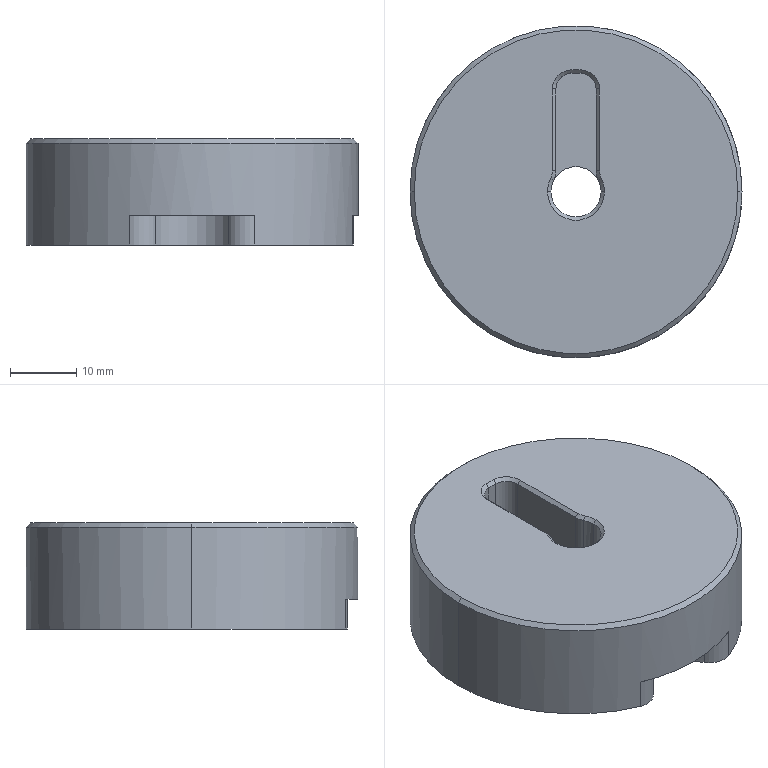NC program | NX | posted with a generic post | part box 50.292 x 50.292 x 16.057 mm
Whole program:
N10 G17 G21 G94 G90
(DRILLING_COPY_1 , TOOL : ZXZ)
N12 T01 M6
N14 G54
N16 G17 G0 G90 X13.47 Y13.47 S3000 M3
N18 G43 Z30. H1
N20 G94 G81 G98 Z-1. F200. R3.
N22 X0. Y-12.898
N24 X-13.47 Y-13.47
N26 G80
N28 G0 X-13.47 Y-13.47 Z30.
N30 M5
(FLOOR_WALL_1 , TOOL : D4)
N32 T04 M6
N34 G54
N36 G17 G0 G90 X4.162 Y28.342 S4000 M3
N38 G43 Z30. H4
N40 Z1.329
N42 G94 G1 Z-0.171 F1800.
N44 X4.655 Y26.949
N46 G3 X4.959 Y26.689 R0.4
N48 G2 X15.213 Y22.483 R27.146
N50 G1 X15.207 Y22.475
N52 G3 X9.475 Y21.472 R5.275
N54 G1 X0.193 Y12.694
N56 G2 X-0.281 Y12.898 R0.281
N58 G1 Y21.257
N60 G3 X-5.704 Y26.53 R5.275
N62 G1 X-5.706 Y26.54
N64 G2 X4.959 Y26.689 R27.146
N66 G1 X4.593 Y24.723
N68 G2 X8.844 Y23.54 R25.146
N70 G3 X8.1 Y22.925 R7.275
N72 G1 X1.719 Y16.889
N74 Y21.257
N76 G3 X0.596 Y25.139 R7.275
N78 G2 X4.593 Y24.723 R25.146
N80 G1 X4.228 Y22.757
N82 G2 X4.875 Y22.627 R23.146
N84 G1 X3.715 Y21.53
N86 G3 X3.578 Y22.868 R9.275
N88 G2 X4.228 Y22.757 R23.146
N90 G3 X4.605 Y22.89 R0.4
N92 G1 Z1.329
N94 G0 X4.162 Y28.342 Z1.135
N96 G1 Z-0.365
N98 X4.655 Y26.949
N100 G3 X4.959 Y26.689 R0.4
N102 G2 X15.213 Y22.483 R27.146
N104 G1 X15.207 Y22.475
N106 G3 X9.475 Y21.472 R5.275
N108 G1 X0.193 Y12.694
N110 G2 X-0.281 Y12.898 R0.281
N112 G1 Y21.257
N114 G3 X-5.704 Y26.53 R5.275
N116 G1 X-5.706 Y26.54
N118 G2 X4.959 Y26.689 R27.146
N120 G1 X4.593 Y24.723
N122 G2 X8.844 Y23.54 R25.146
N124 G3 X8.1 Y22.925 R7.275
N126 G1 X1.719 Y16.889
N128 Y21.257
N130 G3 X0.596 Y25.139 R7.275
N132 G2 X4.593 Y24.723 R25.146
N134 G1 X4.228 Y22.757
N136 G2 X4.875 Y22.627 R23.146
N138 G1 X3.715 Y21.53
N140 G3 X3.578 Y22.868 R9.275
N142 G2 X4.228 Y22.757 R23.146
N144 G3 X4.605 Y22.89 R0.4
N146 G1 Z1.135
N148 G0 X4.162 Y28.342 Z0.942
N150 G1 Z-0.558
N152 X4.655 Y26.949
N154 G3 X4.959 Y26.689 R0.4
N156 G2 X15.213 Y22.483 R27.146
N158 G1 X15.207 Y22.475
N160 G3 X9.475 Y21.472 R5.275
N162 G1 X0.193 Y12.694
N164 G2 X-0.281 Y12.898 R0.281
N166 G1 Y21.257
N168 G3 X-5.704 Y26.53 R5.275
N170 G1 X-5.706 Y26.54
N172 G2 X4.959 Y26.689 R27.146
N174 G1 X4.593 Y24.723
N176 G2 X8.844 Y23.54 R25.146
N178 G3 X8.1 Y22.925 R7.275
N180 G1 X1.719 Y16.889
N182 Y21.257
N184 G3 X0.596 Y25.139 R7.275
N186 G2 X4.593 Y24.723 R25.146
N188 G1 X4.228 Y22.757
N190 G2 X4.875 Y22.627 R23.146
N192 G1 X3.715 Y21.53
N194 G3 X3.578 Y22.868 R9.275
N196 G2 X4.228 Y22.757 R23.146
N198 G3 X4.605 Y22.89 R0.4
N200 G1 Z0.942
N202 G0 X4.162 Y28.342 Z0.748
N204 G1 Z-0.752
N206 X4.655 Y26.949
N208 G3 X4.959 Y26.689 R0.4
N210 G2 X15.213 Y22.483 R27.146
N212 G1 X15.207 Y22.475
N214 G3 X9.475 Y21.472 R5.275
N216 G1 X0.193 Y12.694
N218 G2 X-0.281 Y12.898 R0.281
N220 G1 Y21.257
N222 G3 X-5.704 Y26.53 R5.275
N224 G1 X-5.706 Y26.54
N226 G2 X4.959 Y26.689 R27.146
N228 G1 X4.593 Y24.723
N230 G2 X8.844 Y23.54 R25.146
N232 G3 X8.1 Y22.925 R7.275
N234 G1 X1.719 Y16.889
N236 Y21.257
N238 G3 X0.596 Y25.139 R7.275
N240 G2 X4.593 Y24.723 R25.146
N242 G1 X4.228 Y22.757
N244 G2 X4.875 Y22.627 R23.146
N246 G1 X3.715 Y21.53
N248 G3 X3.578 Y22.868 R9.275
N250 G2 X4.228 Y22.757 R23.146
N252 G3 X4.605 Y22.89 R0.4
N254 G1 Z0.748
N256 G0 X4.162 Y28.342 Z0.555
N258 G1 Z-0.945
N260 X4.655 Y26.949
N262 G3 X4.959 Y26.689 R0.4
N264 G2 X15.213 Y22.483 R27.146
N266 G1 X15.207 Y22.475
N268 G3 X9.475 Y21.472 R5.275
N270 G1 X0.193 Y12.694
N272 G2 X-0.281 Y12.898 R0.281
N274 G1 Y21.257
N276 G3 X-5.704 Y26.53 R5.275
N278 G1 X-5.706 Y26.54
N280 G2 X4.959 Y26.689 R27.146
N282 G1 X4.593 Y24.723
N284 G2 X8.844 Y23.54 R25.146
N286 G3 X8.1 Y22.925 R7.275
N288 G1 X1.719 Y16.889
N290 Y21.257
N292 G3 X0.596 Y25.139 R7.275
N294 G2 X4.593 Y24.723 R25.146
N296 G1 X4.228 Y22.757
N298 G2 X4.875 Y22.627 R23.146
N300 G1 X3.715 Y21.53
N302 G3 X3.578 Y22.868 R9.275
N304 G2 X4.228 Y22.757 R23.146
N306 G3 X4.605 Y22.89 R0.4
N308 G1 Z0.555
N310 G0 X4.162 Y28.342 Z0.361
N312 G1 Z-1.139
N314 X4.655 Y26.949
N316 G3 X4.959 Y26.689 R0.4
N318 G2 X15.213 Y22.483 R27.146
N320 G1 X15.207 Y22.475
N322 G3 X9.475 Y21.472 R5.275
N324 G1 X0.193 Y12.694
N326 G2 X-0.281 Y12.898 R0.281
N328 G1 Y21.257
N330 G3 X-5.704 Y26.53 R5.275
N332 G1 X-5.706 Y26.54
N334 G2 X4.959 Y26.689 R27.146
N336 G1 X4.593 Y24.723
N338 G2 X8.844 Y23.54 R25.146
N340 G3 X8.1 Y22.925 R7.275
N342 G1 X1.719 Y16.889
N344 Y21.257
N346 G3 X0.596 Y25.139 R7.275
N348 G2 X4.593 Y24.723 R25.146
N350 G1 X4.228 Y22.757
N352 G2 X4.875 Y22.627 R23.146
N354 G1 X3.715 Y21.53
N356 G3 X3.578 Y22.868 R9.275
N358 G2 X4.228 Y22.757 R23.146
N360 G3 X4.605 Y22.89 R0.4
N362 G1 Z0.361
N364 G0 X4.162 Y28.342 Z0.168
N366 G1 Z-1.332
N368 X4.655 Y26.949
N370 G3 X4.959 Y26.689 R0.4
N372 G2 X15.213 Y22.483 R27.146
N374 G1 X15.207 Y22.475
N376 G3 X9.475 Y21.472 R5.275
N378 G1 X0.193 Y12.694
N380 G2 X-0.281 Y12.898 R0.281
N382 G1 Y21.257
N384 G3 X-5.704 Y26.53 R5.275
N386 G1 X-5.706 Y26.54
N388 G2 X4.959 Y26.689 R27.146
N390 G1 X4.593 Y24.723
N392 G2 X8.844 Y23.54 R25.146
N394 G3 X8.1 Y22.925 R7.275
N396 G1 X1.719 Y16.889
N398 Y21.257
N400 G3 X0.596 Y25.139 R7.275
N402 G2 X4.593 Y24.723 R25.146
N404 G1 X4.228 Y22.757
N406 G2 X4.875 Y22.627 R23.146
N408 G1 X3.715 Y21.53
N410 G3 X3.578 Y22.868 R9.275
N412 G2 X4.228 Y22.757 R23.146
N414 G3 X4.605 Y22.89 R0.4
N416 G1 Z0.168
N418 G0 X4.162 Y28.342 Z-0.026
N420 G1 Z-1.526
N422 X4.655 Y26.949
N424 G3 X4.959 Y26.689 R0.4
N426 G2 X15.213 Y22.483 R27.146
N428 G1 X15.207 Y22.475
N430 G3 X9.475 Y21.472 R5.275
N432 G1 X0.193 Y12.694
N434 G2 X-0.281 Y12.898 R0.281
N436 G1 Y21.257
N438 G3 X-5.704 Y26.53 R5.275
N440 G1 X-5.706 Y26.54
N442 G2 X4.959 Y26.689 R27.146
N444 G1 X4.593 Y24.723
N446 G2 X8.844 Y23.54 R25.146
N448 G3 X8.1 Y22.925 R7.275
N450 G1 X1.719 Y16.889
N452 Y21.257
N454 G3 X0.596 Y25.139 R7.275
N456 G2 X4.593 Y24.723 R25.146
N458 G1 X4.228 Y22.757
N460 G2 X4.875 Y22.627 R23.146
N462 G1 X3.715 Y21.53
N464 G3 X3.578 Y22.868 R9.275
N466 G2 X4.228 Y22.757 R23.146
N468 G3 X4.605 Y22.89 R0.4
N470 G1 Z-0.026
N472 G0 X4.162 Y28.342 Z-0.219
N474 G1 Z-1.719
N476 X4.655 Y26.949
N478 G3 X4.959 Y26.689 R0.4
N480 G2 X15.213 Y22.483 R27.146
N482 G1 X15.207 Y22.475
N484 G3 X9.475 Y21.472 R5.275
N486 G1 X0.193 Y12.694
N488 G2 X-0.281 Y12.898 R0.281
N490 G1 Y21.257
N492 G3 X-5.704 Y26.53 R5.275
N494 G1 X-5.706 Y26.54
N496 G2 X4.959 Y26.689 R27.146
N498 G1 X4.593 Y24.723
N500 G2 X8.844 Y23.54 R25.146
N502 G3 X8.1 Y22.925 R7.275
N504 G1 X1.719 Y16.889
N506 Y21.257
N508 G3 X0.596 Y25.139 R7.275
N510 G2 X4.593 Y24.723 R25.146
N512 G1 X4.228 Y22.757
N514 G2 X4.875 Y22.627 R23.146
N516 G1 X3.715 Y21.53
N518 G3 X3.578 Y22.868 R9.275
N520 G2 X4.228 Y22.757 R23.146
N522 G3 X4.605 Y22.89 R0.4
N524 G1 Z-0.219
N526 G0 X4.162 Y28.342 Z-0.413
N528 G1 Z-1.913
N530 X4.655 Y26.949
N532 G3 X4.959 Y26.689 R0.4
N534 G2 X15.213 Y22.483 R27.146
N536 G1 X15.207 Y22.475
N538 G3 X9.475 Y21.472 R5.275
N540 G1 X0.193 Y12.694
N542 G2 X-0.281 Y12.898 R0.281
N544 G1 Y21.257
N546 G3 X-5.704 Y26.53 R5.275
N548 G1 X-5.706 Y26.54
N550 G2 X4.959 Y26.689 R27.146
N552 G1 X4.593 Y24.723
N554 G2 X8.844 Y23.54 R25.146
N556 G3 X8.1 Y22.925 R7.275
N558 G1 X1.719 Y16.889
N560 Y21.257
N562 G3 X0.596 Y25.139 R7.275
N564 G2 X4.593 Y24.723 R25.146
N566 G1 X4.228 Y22.757
N568 G2 X4.875 Y22.627 R23.146
N570 G1 X3.715 Y21.53
N572 G3 X3.578 Y22.868 R9.275
N574 G2 X4.228 Y22.757 R23.146
N576 G3 X4.605 Y22.89 R0.4
N578 G1 Z-0.413
N580 G0 X4.162 Y28.342 Z-0.606
N582 G1 Z-2.106
N584 X4.655 Y26.949
N586 G3 X4.959 Y26.689 R0.4
N588 G2 X15.213 Y22.483 R27.146
N590 G1 X15.207 Y22.475
N592 G3 X9.475 Y21.472 R5.275
N594 G1 X0.193 Y12.694
N596 G2 X-0.281 Y12.898 R0.281
N598 G1 Y21.257
N600 G3 X-5.704 Y26.53 R5.275
N602 G1 X-5.706 Y26.54
N604 G2 X4.959 Y26.689 R27.146
N606 G1 X4.593 Y24.723
N608 G2 X8.844 Y23.54 R25.146
N610 G3 X8.1 Y22.925 R7.275
N612 G1 X1.719 Y16.889
N614 Y21.257
N616 G3 X0.596 Y25.139 R7.275
N618 G2 X4.593 Y24.723 R25.146
N620 G1 X4.228 Y22.757
N622 G2 X4.875 Y22.627 R23.146
N624 G1 X3.715 Y21.53
N626 G3 X3.578 Y22.868 R9.275
N628 G2 X4.228 Y22.757 R23.146
N630 G3 X4.605 Y22.89 R0.4
N632 G1 Z-0.606
N634 G0 X4.162 Y28.342 Z-0.8
N636 G1 Z-2.3
N638 X4.655 Y26.949
N640 G3 X4.959 Y26.689 R0.4
N642 G2 X15.213 Y22.483 R27.146
N644 G1 X15.207 Y22.475
N646 G3 X9.475 Y21.472 R5.275
N648 G1 X0.193 Y12.694
N650 G2 X-0.281 Y12.898 R0.281
N652 G1 Y21.257
N654 G3 X-5.704 Y26.53 R5.275
N656 G1 X-5.706 Y26.54
N658 G2 X4.959 Y26.689 R27.146
N660 G1 X4.593 Y24.723
N662 G2 X8.844 Y23.54 R25.146
N664 G3 X8.1 Y22.925 R7.275
N666 G1 X1.719 Y16.889
N668 Y21.257
N670 G3 X0.596 Y25.139 R7.275
N672 G2 X4.593 Y24.723 R25.146
N674 G1 X4.228 Y22.757
N676 G2 X4.875 Y22.627 R23.146
N678 G1 X3.715 Y21.53
N680 G3 X3.578 Y22.868 R9.275
N682 G2 X4.228 Y22.757 R23.146
N684 G3 X4.605 Y22.89 R0.4
N686 G1 Z-0.8
N688 G0 X4.162 Y28.342 Z-0.993
N690 G1 Z-2.493
N692 X4.655 Y26.949
N694 G3 X4.959 Y26.689 R0.4
N696 G2 X15.213 Y22.483 R27.146
N698 G1 X15.207 Y22.475
N700 G3 X9.475 Y21.472 R5.275
N702 G1 X0.193 Y12.694
N704 G2 X-0.281 Y12.898 R0.281
N706 G1 Y21.257
N708 G3 X-5.704 Y26.53 R5.275
N710 G1 X-5.706 Y26.54
N712 G2 X4.959 Y26.689 R27.146
N714 G1 X4.593 Y24.723
N716 G2 X8.844 Y23.54 R25.146
N718 G3 X8.1 Y22.925 R7.275
N720 G1 X1.719 Y16.889
N722 Y21.257
N724 G3 X0.596 Y25.139 R7.275
N726 G2 X4.593 Y24.723 R25.146
N728 G1 X4.228 Y22.757
N730 G2 X4.875 Y22.627 R23.146
N732 G1 X3.715 Y21.53
N734 G3 X3.578 Y22.868 R9.275
N736 G2 X4.228 Y22.757 R23.146
N738 G3 X4.605 Y22.89 R0.4
N740 G1 Z-0.993
N742 G0 X4.162 Y28.342 Z-1.187
N744 G1 Z-2.687
N746 X4.655 Y26.949
N748 G3 X4.959 Y26.689 R0.4
N750 G2 X15.213 Y22.483 R27.146
N752 G1 X15.207 Y22.475
N754 G3 X9.475 Y21.472 R5.275
N756 G1 X0.193 Y12.694
N758 G2 X-0.281 Y12.898 R0.281
N760 G1 Y21.257
N762 G3 X-5.704 Y26.53 R5.275
N764 G1 X-5.706 Y26.54
N766 G2 X4.959 Y26.689 R27.146
N768 G1 X4.593 Y24.723
N770 G2 X8.844 Y23.54 R25.146
N772 G3 X8.1 Y22.925 R7.275
N774 G1 X1.719 Y16.889
N776 Y21.257
N778 G3 X0.596 Y25.139 R7.275
N780 G2 X4.593 Y24.723 R25.146
N782 G1 X4.228 Y22.757
N784 G2 X4.875 Y22.627 R23.146
N786 G1 X3.715 Y21.53
N788 G3 X3.578 Y22.868 R9.275
N790 G2 X4.228 Y22.757 R23.146
N792 G3 X4.605 Y22.89 R0.4
N794 G1 Z-1.187
N796 G0 X4.162 Y28.342 Z-1.38
N798 G1 Z-2.88
N800 X4.655 Y26.949
N802 G3 X4.959 Y26.689 R0.4
N804 G2 X15.213 Y22.483 R27.146
N806 G1 X15.207 Y22.475
N808 G3 X9.475 Y21.472 R5.275
N810 G1 X0.193 Y12.694
N812 G2 X-0.281 Y12.898 R0.281
N814 G1 Y21.257
N816 G3 X-5.704 Y26.53 R5.275
N818 G1 X-5.706 Y26.54
N820 G2 X4.959 Y26.689 R27.146
N822 G1 X4.593 Y24.723
N824 G2 X8.844 Y23.54 R25.146
N826 G3 X8.1 Y22.925 R7.275
N828 G1 X1.719 Y16.889
N830 Y21.257
N832 G3 X0.596 Y25.139 R7.275
N834 G2 X4.593 Y24.723 R25.146
N836 G1 X4.228 Y22.757
N838 G2 X4.875 Y22.627 R23.146
N840 G1 X3.715 Y21.53
N842 G3 X3.578 Y22.868 R9.275
N844 G2 X4.228 Y22.757 R23.146
N846 G3 X4.605 Y22.89 R0.4
N848 G1 Z-1.38
N850 G0 X4.162 Y28.342 Z-1.574
N852 G1 Z-3.074
N854 X4.655 Y26.949
N856 G3 X4.959 Y26.689 R0.4
N858 G2 X15.213 Y22.483 R27.146
N860 G1 X15.207 Y22.475
N862 G3 X9.475 Y21.472 R5.275
N864 G1 X0.193 Y12.694
N866 G2 X-0.281 Y12.898 R0.281
N868 G1 Y21.257
N870 G3 X-5.704 Y26.53 R5.275
N872 G1 X-5.706 Y26.54
N874 G2 X4.959 Y26.689 R27.146
N876 G1 X4.593 Y24.723
N878 G2 X8.844 Y23.54 R25.146
N880 G3 X8.1 Y22.925 R7.275
N882 G1 X1.719 Y16.889
N884 Y21.257
N886 G3 X0.596 Y25.139 R7.275
N888 G2 X4.593 Y24.723 R25.146
N890 G1 X4.228 Y22.757
N892 G2 X4.875 Y22.627 R23.146
N894 G1 X3.715 Y21.53
N896 G3 X3.578 Y22.868 R9.275
N898 G2 X4.228 Y22.757 R23.146
N900 G3 X4.605 Y22.89 R0.4
N902 G1 Z-1.574
N904 G0 X4.162 Y28.342 Z-1.767
N906 G1 Z-3.267
N908 X4.655 Y26.949
N910 G3 X4.959 Y26.689 R0.4
N912 G2 X15.213 Y22.483 R27.146
N914 G1 X15.207 Y22.475
N916 G3 X9.475 Y21.472 R5.275
N918 G1 X0.193 Y12.694
N920 G2 X-0.281 Y12.898 R0.281
N922 G1 Y21.257
N924 G3 X-5.704 Y26.53 R5.275
N926 G1 X-5.706 Y26.54
N928 G2 X4.959 Y26.689 R27.146
N930 G1 X4.593 Y24.723
N932 G2 X8.844 Y23.54 R25.146
N934 G3 X8.1 Y22.925 R7.275
N936 G1 X1.719 Y16.889
N938 Y21.257
N940 G3 X0.596 Y25.139 R7.275
N942 G2 X4.593 Y24.723 R25.146
N944 G1 X4.228 Y22.757
N946 G2 X4.875 Y22.627 R23.146
N948 G1 X3.715 Y21.53
N950 G3 X3.578 Y22.868 R9.275
N952 G2 X4.228 Y22.757 R23.146
N954 G3 X4.605 Y22.89 R0.4
N956 G1 Z-1.767
N958 G0 X4.162 Y28.342 Z-1.961
N960 G1 Z-3.461
N962 X4.655 Y26.949
N964 G3 X4.959 Y26.689 R0.4
N966 G2 X15.213 Y22.483 R27.146
N968 G1 X15.207 Y22.475
N970 G3 X9.475 Y21.472 R5.275
N972 G1 X0.193 Y12.694
N974 G2 X-0.281 Y12.898 R0.281
N976 G1 Y21.257
N978 G3 X-5.704 Y26.53 R5.275
N980 G1 X-5.706 Y26.54
N982 G2 X4.959 Y26.689 R27.146
N984 G1 X4.593 Y24.723
N986 G2 X8.844 Y23.54 R25.146
N988 G3 X8.1 Y22.925 R7.275
N990 G1 X1.719 Y16.889
N992 Y21.257
N994 G3 X0.596 Y25.139 R7.275
N996 G2 X4.593 Y24.723 R25.146
N998 G1 X4.228 Y22.757
N1000 G2 X4.875 Y22.627 R23.146
N1002 G1 X3.715 Y21.53
N1004 G3 X3.578 Y22.868 R9.275
N1006 G2 X4.228 Y22.757 R23.146
N1008 G3 X4.605 Y22.89 R0.4
N1010 G1 Z-1.961
N1012 G0 X4.162 Y28.342 Z-2.154
N1014 G1 Z-3.654
N1016 X4.655 Y26.949
N1018 G3 X4.959 Y26.689 R0.4
N1020 G2 X15.213 Y22.483 R27.146
N1022 G1 X15.207 Y22.475
N1024 G3 X9.475 Y21.472 R5.275
N1026 G1 X0.193 Y12.694
N1028 G2 X-0.281 Y12.898 R0.281
N1030 G1 Y21.257
N1032 G3 X-5.704 Y26.53 R5.275
N1034 G1 X-5.706 Y26.54
N1036 G2 X4.959 Y26.689 R27.146
N1038 G1 X4.593 Y24.723
N1040 G2 X8.844 Y23.54 R25.146
N1042 G3 X8.1 Y22.925 R7.275
N1044 G1 X1.719 Y16.889
N1046 Y21.257
N1048 G3 X0.596 Y25.139 R7.275
N1050 G2 X4.593 Y24.723 R25.146
N1052 G1 X4.228 Y22.757
N1054 G2 X4.875 Y22.627 R23.146
N1056 G1 X3.715 Y21.53
N1058 G3 X3.578 Y22.868 R9.275
N1060 G2 X4.228 Y22.757 R23.146
N1062 G3 X4.605 Y22.89 R0.4
N1064 G1 Z-2.154
N1066 G0 X4.162 Y28.342 Z-2.348
N1068 G1 Z-3.848
N1070 X4.655 Y26.949
N1072 G3 X4.959 Y26.689 R0.4
N1074 G2 X15.213 Y22.483 R27.146
N1076 G1 X15.207 Y22.475
N1078 G3 X9.475 Y21.472 R5.275
N1080 G1 X0.193 Y12.694
N1082 G2 X-0.281 Y12.898 R0.281
N1084 G1 Y21.257
N1086 G3 X-5.704 Y26.53 R5.275
N1088 G1 X-5.706 Y26.54
N1090 G2 X4.959 Y26.689 R27.146
N1092 G1 X4.593 Y24.723
N1094 G2 X8.844 Y23.54 R25.146
N1096 G3 X8.1 Y22.925 R7.275
N1098 G1 X1.719 Y16.889
N1100 Y21.257
N1102 G3 X0.596 Y25.139 R7.275
N1104 G2 X4.593 Y24.723 R25.146
N1106 G1 X4.228 Y22.757
N1108 G2 X4.875 Y22.627 R23.146
N1110 G1 X3.715 Y21.53
N1112 G3 X3.578 Y22.868 R9.275
N1114 G2 X4.228 Y22.757 R23.146
N1116 G3 X4.605 Y22.89 R0.4
N1118 G1 Z-2.348
N1120 G0 X4.162 Y28.342 Z-2.541
N1122 G1 Z-4.041
N1124 X4.655 Y26.949
N1126 G3 X4.959 Y26.689 R0.4
N1128 G2 X15.213 Y22.483 R27.146
N1130 G1 X15.207 Y22.475
N1132 G3 X9.475 Y21.472 R5.275
N1134 G1 X0.193 Y12.694
N1136 G2 X-0.281 Y12.898 R0.281
N1138 G1 Y21.257
N1140 G3 X-5.704 Y26.53 R5.275
N1142 G1 X-5.706 Y26.54
N1144 G2 X4.959 Y26.689 R27.146
N1146 G1 X4.593 Y24.723
N1148 G2 X8.844 Y23.54 R25.146
N1150 G3 X8.1 Y22.925 R7.275
N1152 G1 X1.719 Y16.889
N1154 Y21.257
N1156 G3 X0.596 Y25.139 R7.275
N1158 G2 X4.593 Y24.723 R25.146
N1160 G1 X4.228 Y22.757
N1162 G2 X4.875 Y22.627 R23.146
N1164 G1 X3.715 Y21.53
N1166 G3 X3.578 Y22.868 R9.275
N1168 G2 X4.228 Y22.757 R23.146
N1170 G3 X4.605 Y22.89 R0.4
N1172 G1 Z-2.541
N1174 G0 X4.162 Y28.342 Z-2.735
N1176 G1 Z-4.235
N1178 X4.655 Y26.949
N1180 G3 X4.959 Y26.689 R0.4
N1182 G2 X15.213 Y22.483 R27.146
N1184 G1 X15.207 Y22.475
N1186 G3 X9.475 Y21.472 R5.275
N1188 G1 X0.193 Y12.694
N1190 G2 X-0.281 Y12.898 R0.281
N1192 G1 Y21.257
N1194 G3 X-5.704 Y26.53 R5.275
N1196 G1 X-5.706 Y26.54
N1198 G2 X4.959 Y26.689 R27.146
N1200 G1 X4.593 Y24.723
N1202 G2 X8.844 Y23.54 R25.146
N1204 G3 X8.1 Y22.925 R7.275
N1206 G1 X1.719 Y16.889
N1208 Y21.257
N1210 G3 X0.596 Y25.139 R7.275
N1212 G2 X4.593 Y24.723 R25.146
N1214 G1 X4.228 Y22.757
N1216 G2 X4.875 Y22.627 R23.146
N1218 G1 X3.715 Y21.53
N1220 G3 X3.578 Y22.868 R9.275
N1222 G2 X4.228 Y22.757 R23.146
N1224 G3 X4.605 Y22.89 R0.4
N1226 G1 Z-2.735
N1228 G0 X4.162 Y28.342 Z-2.928
N1230 G1 Z-4.428
N1232 X4.655 Y26.949
N1234 G3 X4.959 Y26.689 R0.4
N1236 G2 X15.213 Y22.483 R27.146
N1238 G1 X15.207 Y22.475
N1240 G3 X9.475 Y21.472 R5.275
N1242 G1 X0.193 Y12.694
N1244 G2 X-0.281 Y12.898 R0.281
N1246 G1 Y21.257
N1248 G3 X-5.704 Y26.53 R5.275
N1250 G1 X-5.706 Y26.54
N1252 G2 X4.959 Y26.689 R27.146
N1254 G1 X4.593 Y24.723
N1256 G2 X8.844 Y23.54 R25.146
N1258 G3 X8.1 Y22.925 R7.275
N1260 G1 X1.719 Y16.889
N1262 Y21.257
N1264 G3 X0.596 Y25.139 R7.275
N1266 G2 X4.593 Y24.723 R25.146
N1268 G1 X4.228 Y22.757
N1270 G2 X4.875 Y22.627 R23.146
N1272 G1 X3.715 Y21.53
N1274 G3 X3.578 Y22.868 R9.275
N1276 G2 X4.228 Y22.757 R23.146
N1278 G3 X4.605 Y22.89 R0.4
N1280 G1 Z-2.928
N1282 G0 Z30.
N1284 X-28.625 Y-1.085
N1286 Z1.329
N1288 G1 Z-0.171
N1290 X-27.346 Y-0.346
N1292 G3 X-27.146 Y0. R0.4
N1294 G2 X-25.574 Y9.104 R27.146
N1296 G1 X-25.565 Y9.1
N1298 G3 X-22.973 Y3.69 R5.275
N1300 G2 X-22.973 Y-3.69 R4.25
N1302 G3 X-25.565 Y-9.1 R5.275
N1304 G1 X-25.574 Y-9.104
N1306 G2 X-27.146 Y0. R27.146
N1308 G1 X-25.146
N1310 G2 X-25.004 Y2.673 R25.146
N1312 G3 X-23.966 Y1.953 R7.275
N1314 G2 X-23.966 Y-1.953 R2.25
N1316 G3 X-25.004 Y-2.673 R7.275
N1318 G2 X-25.146 Y0. R25.146
N1320 G3 X-25.346 Y0.346 R0.4
N1322 G1 X-28.643 Y0.391
N1324 Z1.329
N1326 G0 X-28.625 Y-1.085 Z1.135
N1328 G1 Z-0.365
N1330 X-27.346 Y-0.346
N1332 G3 X-27.146 Y0. R0.4
N1334 G2 X-25.574 Y9.104 R27.146
N1336 G1 X-25.565 Y9.1
N1338 G3 X-22.973 Y3.69 R5.275
N1340 G2 X-22.973 Y-3.69 R4.25
N1342 G3 X-25.565 Y-9.1 R5.275
N1344 G1 X-25.574 Y-9.104
N1346 G2 X-27.146 Y0. R27.146
N1348 G1 X-25.146
N1350 G2 X-25.004 Y2.673 R25.146
N1352 G3 X-23.966 Y1.953 R7.275
N1354 G2 X-23.966 Y-1.953 R2.25
N1356 G3 X-25.004 Y-2.673 R7.275
N1358 G2 X-25.146 Y0. R25.146
N1360 G3 X-25.346 Y0.346 R0.4
N1362 G1 X-28.643 Y0.391
N1364 Z1.135
N1366 G0 X-28.625 Y-1.085 Z0.942
N1368 G1 Z-0.558
N1370 X-27.346 Y-0.346
N1372 G3 X-27.146 Y0. R0.4
N1374 G2 X-25.574 Y9.104 R27.146
N1376 G1 X-25.565 Y9.1
N1378 G3 X-22.973 Y3.69 R5.275
N1380 G2 X-22.973 Y-3.69 R4.25
N1382 G3 X-25.565 Y-9.1 R5.275
N1384 G1 X-25.574 Y-9.104
N1386 G2 X-27.146 Y0. R27.146
N1388 G1 X-25.146
N1390 G2 X-25.004 Y2.673 R25.146
N1392 G3 X-23.966 Y1.953 R7.275
N1394 G2 X-23.966 Y-1.953 R2.25
N1396 G3 X-25.004 Y-2.673 R7.275
N1398 G2 X-25.146 Y0. R25.146
N1400 G3 X-25.346 Y0.346 R0.4
N1402 G1 X-28.643 Y0.391
N1404 Z0.942
N1406 G0 X-28.625 Y-1.085 Z0.748
N1408 G1 Z-0.752
N1410 X-27.346 Y-0.346
N1412 G3 X-27.146 Y0. R0.4
N1414 G2 X-25.574 Y9.104 R27.146
N1416 G1 X-25.565 Y9.1
N1418 G3 X-22.973 Y3.69 R5.275
N1420 G2 X-22.973 Y-3.69 R4.25
N1422 G3 X-25.565 Y-9.1 R5.275
N1424 G1 X-25.574 Y-9.104
N1426 G2 X-27.146 Y0. R27.146
N1428 G1 X-25.146
N1430 G2 X-25.004 Y2.673 R25.146
N1432 G3 X-23.966 Y1.953 R7.275
N1434 G2 X-23.966 Y-1.953 R2.25
N1436 G3 X-25.004 Y-2.673 R7.275
N1438 G2 X-25.146 Y0. R25.146
N1440 G3 X-25.346 Y0.346 R0.4
N1442 G1 X-28.643 Y0.391
N1444 Z0.748
N1446 G0 X-28.625 Y-1.085 Z0.555
N1448 G1 Z-0.945
N1450 X-27.346 Y-0.346
N1452 G3 X-27.146 Y0. R0.4
N1454 G2 X-25.574 Y9.104 R27.146
N1456 G1 X-25.565 Y9.1
N1458 G3 X-22.973 Y3.69 R5.275
N1460 G2 X-22.973 Y-3.69 R4.25
N1462 G3 X-25.565 Y-9.1 R5.275
N1464 G1 X-25.574 Y-9.104
N1466 G2 X-27.146 Y0. R27.146
N1468 G1 X-25.146
N1470 G2 X-25.004 Y2.673 R25.146
N1472 G3 X-23.966 Y1.953 R7.275
N1474 G2 X-23.966 Y-1.953 R2.25
N1476 G3 X-25.004 Y-2.673 R7.275
N1478 G2 X-25.146 Y0. R25.146
N1480 G3 X-25.346 Y0.346 R0.4
N1482 G1 X-28.643 Y0.391
N1484 Z0.555
N1486 G0 X-28.625 Y-1.085 Z0.361
N1488 G1 Z-1.139
N1490 X-27.346 Y-0.346
N1492 G3 X-27.146 Y0. R0.4
N1494 G2 X-25.574 Y9.104 R27.146
N1496 G1 X-25.565 Y9.1
N1498 G3 X-22.973 Y3.69 R5.275
N1500 G2 X-22.973 Y-3.69 R4.25
N1502 G3 X-25.565 Y-9.1 R5.275
N1504 G1 X-25.574 Y-9.104
N1506 G2 X-27.146 Y0. R27.146
N1508 G1 X-25.146
N1510 G2 X-25.004 Y2.673 R25.146
N1512 G3 X-23.966 Y1.953 R7.275
N1514 G2 X-23.966 Y-1.953 R2.25
N1516 G3 X-25.004 Y-2.673 R7.275
N1518 G2 X-25.146 Y0. R25.146
N1520 G3 X-25.346 Y0.346 R0.4
N1522 G1 X-28.643 Y0.391
N1524 Z0.361
N1526 G0 X-28.625 Y-1.085 Z0.168
N1528 G1 Z-1.332
N1530 X-27.346 Y-0.346
N1532 G3 X-27.146 Y0. R0.4
N1534 G2 X-25.574 Y9.104 R27.146
N1536 G1 X-25.565 Y9.1
N1538 G3 X-22.973 Y3.69 R5.275
N1540 G2 X-22.973 Y-3.69 R4.25
N1542 G3 X-25.565 Y-9.1 R5.275
N1544 G1 X-25.574 Y-9.104
N1546 G2 X-27.146 Y0. R27.146
N1548 G1 X-25.146
N1550 G2 X-25.004 Y2.673 R25.146
N1552 G3 X-23.966 Y1.953 R7.275
N1554 G2 X-23.966 Y-1.953 R2.25
N1556 G3 X-25.004 Y-2.673 R7.275
N1558 G2 X-25.146 Y0. R25.146
N1560 G3 X-25.346 Y0.346 R0.4
N1562 G1 X-28.643 Y0.391
N1564 Z0.168
N1566 G0 X-28.625 Y-1.085 Z-0.026
N1568 G1 Z-1.526
N1570 X-27.346 Y-0.346
N1572 G3 X-27.146 Y0. R0.4
N1574 G2 X-25.574 Y9.104 R27.146
N1576 G1 X-25.565 Y9.1
N1578 G3 X-22.973 Y3.69 R5.275
N1580 G2 X-22.973 Y-3.69 R4.25
N1582 G3 X-25.565 Y-9.1 R5.275
N1584 G1 X-25.574 Y-9.104
N1586 G2 X-27.146 Y0. R27.146
N1588 G1 X-25.146
N1590 G2 X-25.004 Y2.673 R25.146
N1592 G3 X-23.966 Y1.953 R7.275
N1594 G2 X-23.966 Y-1.953 R2.25
N1596 G3 X-25.004 Y-2.673 R7.275
N1598 G2 X-25.146 Y0. R25.146
N1600 G3 X-25.346 Y0.346 R0.4
N1602 G1 X-28.643 Y0.391
N1604 Z-0.026
N1606 G0 X-28.625 Y-1.085 Z-0.219
N1608 G1 Z-1.719
N1610 X-27.346 Y-0.346
N1612 G3 X-27.146 Y0. R0.4
N1614 G2 X-25.574 Y9.104 R27.146
N1616 G1 X-25.565 Y9.1
N1618 G3 X-22.973 Y3.69 R5.275
N1620 G2 X-22.973 Y-3.69 R4.25
N1622 G3 X-25.565 Y-9.1 R5.275
N1624 G1 X-25.574 Y-9.104
N1626 G2 X-27.146 Y0. R27.146
N1628 G1 X-25.146
N1630 G2 X-25.004 Y2.673 R25.146
N1632 G3 X-23.966 Y1.953 R7.275
N1634 G2 X-23.966 Y-1.953 R2.25
N1636 G3 X-25.004 Y-2.673 R7.275
N1638 G2 X-25.146 Y0. R25.146
N1640 G3 X-25.346 Y0.346 R0.4
N1642 G1 X-28.643 Y0.391
N1644 Z-0.219
N1646 G0 X-28.625 Y-1.085 Z-0.413
N1648 G1 Z-1.913
N1650 X-27.346 Y-0.346
N1652 G3 X-27.146 Y0. R0.4
N1654 G2 X-25.574 Y9.104 R27.146
N1656 G1 X-25.565 Y9.1
N1658 G3 X-22.973 Y3.69 R5.275
N1660 G2 X-22.973 Y-3.69 R4.25
N1662 G3 X-25.565 Y-9.1 R5.275
N1664 G1 X-25.574 Y-9.104
N1666 G2 X-27.146 Y0. R27.146
N1668 G1 X-25.146
N1670 G2 X-25.004 Y2.673 R25.146
N1672 G3 X-23.966 Y1.953 R7.275
N1674 G2 X-23.966 Y-1.953 R2.25
N1676 G3 X-25.004 Y-2.673 R7.275
N1678 G2 X-25.146 Y0. R25.146
N1680 G3 X-25.346 Y0.346 R0.4
N1682 G1 X-28.643 Y0.391
N1684 Z-0.413
N1686 G0 X-28.625 Y-1.085 Z-0.606
N1688 G1 Z-2.106
N1690 X-27.346 Y-0.346
N1692 G3 X-27.146 Y0. R0.4
N1694 G2 X-25.574 Y9.104 R27.146
N1696 G1 X-25.565 Y9.1
N1698 G3 X-22.973 Y3.69 R5.275
N1700 G2 X-22.973 Y-3.69 R4.25
N1702 G3 X-25.565 Y-9.1 R5.275
N1704 G1 X-25.574 Y-9.104
N1706 G2 X-27.146 Y0. R27.146
N1708 G1 X-25.146
N1710 G2 X-25.004 Y2.673 R25.146
N1712 G3 X-23.966 Y1.953 R7.275
N1714 G2 X-23.966 Y-1.953 R2.25
N1716 G3 X-25.004 Y-2.673 R7.275
N1718 G2 X-25.146 Y0. R25.146
N1720 G3 X-25.346 Y0.346 R0.4
N1722 G1 X-28.643 Y0.391
N1724 Z-0.606
N1726 G0 X-28.625 Y-1.085 Z-0.8
N1728 G1 Z-2.3
N1730 X-27.346 Y-0.346
N1732 G3 X-27.146 Y0. R0.4
N1734 G2 X-25.574 Y9.104 R27.146
N1736 G1 X-25.565 Y9.1
N1738 G3 X-22.973 Y3.69 R5.275
N1740 G2 X-22.973 Y-3.69 R4.25
N1742 G3 X-25.565 Y-9.1 R5.275
N1744 G1 X-25.574 Y-9.104
N1746 G2 X-27.146 Y0. R27.146
N1748 G1 X-25.146
N1750 G2 X-25.004 Y2.673 R25.146
N1752 G3 X-23.966 Y1.953 R7.275
N1754 G2 X-23.966 Y-1.953 R2.25
N1756 G3 X-25.004 Y-2.673 R7.275
N1758 G2 X-25.146 Y0. R25.146
N1760 G3 X-25.346 Y0.346 R0.4
N1762 G1 X-28.643 Y0.391
N1764 Z-0.8
N1766 G0 X-28.625 Y-1.085 Z-0.993
N1768 G1 Z-2.493
N1770 X-27.346 Y-0.346
N1772 G3 X-27.146 Y0. R0.4
N1774 G2 X-25.574 Y9.104 R27.146
N1776 G1 X-25.565 Y9.1
N1778 G3 X-22.973 Y3.69 R5.275
N1780 G2 X-22.973 Y-3.69 R4.25
N1782 G3 X-25.565 Y-9.1 R5.275
N1784 G1 X-25.574 Y-9.104
N1786 G2 X-27.146 Y0. R27.146
N1788 G1 X-25.146
N1790 G2 X-25.004 Y2.673 R25.146
N1792 G3 X-23.966 Y1.953 R7.275
N1794 G2 X-23.966 Y-1.953 R2.25
N1796 G3 X-25.004 Y-2.673 R7.275
N1798 G2 X-25.146 Y0. R25.146
N1800 G3 X-25.346 Y0.346 R0.4
N1802 G1 X-28.643 Y0.391
N1804 Z-0.993
N1806 G0 X-28.625 Y-1.085 Z-1.187
N1808 G1 Z-2.687
N1810 X-27.346 Y-0.346
N1812 G3 X-27.146 Y0. R0.4
N1814 G2 X-25.574 Y9.104 R27.146
N1816 G1 X-25.565 Y9.1
N1818 G3 X-22.973 Y3.69 R5.275
N1820 G2 X-22.973 Y-3.69 R4.25
N1822 G3 X-25.565 Y-9.1 R5.275
N1824 G1 X-25.574 Y-9.104
N1826 G2 X-27.146 Y0. R27.146
N1828 G1 X-25.146
N1830 G2 X-25.004 Y2.673 R25.146
N1832 G3 X-23.966 Y1.953 R7.275
N1834 G2 X-23.966 Y-1.953 R2.25
N1836 G3 X-25.004 Y-2.673 R7.275
N1838 G2 X-25.146 Y0. R25.146
N1840 G3 X-25.346 Y0.346 R0.4
N1842 G1 X-28.643 Y0.391
N1844 Z-1.187
N1846 G0 X-28.625 Y-1.085 Z-1.38
N1848 G1 Z-2.88
N1850 X-27.346 Y-0.346
N1852 G3 X-27.146 Y0. R0.4
N1854 G2 X-25.574 Y9.104 R27.146
N1856 G1 X-25.565 Y9.1
N1858 G3 X-22.973 Y3.69 R5.275
N1860 G2 X-22.973 Y-3.69 R4.25
N1862 G3 X-25.565 Y-9.1 R5.275
N1864 G1 X-25.574 Y-9.104
N1866 G2 X-27.146 Y0. R27.146
N1868 G1 X-25.146
N1870 G2 X-25.004 Y2.673 R25.146
N1872 G3 X-23.966 Y1.953 R7.275
N1874 G2 X-23.966 Y-1.953 R2.25
N1876 G3 X-25.004 Y-2.673 R7.275
N1878 G2 X-25.146 Y0. R25.146
N1880 G3 X-25.346 Y0.346 R0.4
N1882 G1 X-28.643 Y0.391
N1884 Z-1.38
N1886 G0 X-28.625 Y-1.085 Z-1.574
N1888 G1 Z-3.074
N1890 X-27.346 Y-0.346
N1892 G3 X-27.146 Y0. R0.4
N1894 G2 X-25.574 Y9.104 R27.146
N1896 G1 X-25.565 Y9.1
N1898 G3 X-22.973 Y3.69 R5.275
N1900 G2 X-22.973 Y-3.69 R4.25
N1902 G3 X-25.565 Y-9.1 R5.275
N1904 G1 X-25.574 Y-9.104
N1906 G2 X-27.146 Y0. R27.146
N1908 G1 X-25.146
N1910 G2 X-25.004 Y2.673 R25.146
N1912 G3 X-23.966 Y1.953 R7.275
N1914 G2 X-23.966 Y-1.953 R2.25
N1916 G3 X-25.004 Y-2.673 R7.275
N1918 G2 X-25.146 Y0. R25.146
N1920 G3 X-25.346 Y0.346 R0.4
N1922 G1 X-28.643 Y0.391
N1924 Z-1.574
N1926 G0 X-28.625 Y-1.085 Z-1.767
N1928 G1 Z-3.267
N1930 X-27.346 Y-0.346
N1932 G3 X-27.146 Y0. R0.4
N1934 G2 X-25.574 Y9.104 R27.146
N1936 G1 X-25.565 Y9.1
N1938 G3 X-22.973 Y3.69 R5.275
N1940 G2 X-22.973 Y-3.69 R4.25
N1942 G3 X-25.565 Y-9.1 R5.275
N1944 G1 X-25.574 Y-9.104
N1946 G2 X-27.146 Y0. R27.146
N1948 G1 X-25.146
N1950 G2 X-25.004 Y2.673 R25.146
N1952 G3 X-23.966 Y1.953 R7.275
N1954 G2 X-23.966 Y-1.953 R2.25
N1956 G3 X-25.004 Y-2.673 R7.275
N1958 G2 X-25.146 Y0. R25.146
N1960 G3 X-25.346 Y0.346 R0.4
N1962 G1 X-28.643 Y0.391
N1964 Z-1.767
N1966 G0 X-28.625 Y-1.085 Z-1.961
N1968 G1 Z-3.461
N1970 X-27.346 Y-0.346
N1972 G3 X-27.146 Y0. R0.4
N1974 G2 X-25.574 Y9.104 R27.146
N1976 G1 X-25.565 Y9.1
N1978 G3 X-22.973 Y3.69 R5.275
N1980 G2 X-22.973 Y-3.69 R4.25
N1982 G3 X-25.565 Y-9.1 R5.275
N1984 G1 X-25.574 Y-9.104
N1986 G2 X-27.146 Y0. R27.146
N1988 G1 X-25.146
N1990 G2 X-25.004 Y2.673 R25.146
N1992 G3 X-23.966 Y1.953 R7.275
N1994 G2 X-23.966 Y-1.953 R2.25
N1996 G3 X-25.004 Y-2.673 R7.275
N1998 G2 X-25.146 Y0. R25.146
N2000 G3 X-25.346 Y0.346 R0.4
N2002 G1 X-28.643 Y0.391
N2004 Z-1.961
N2006 G0 X-28.625 Y-1.085 Z-2.154
N2008 G1 Z-3.654
N2010 X-27.346 Y-0.346
N2012 G3 X-27.146 Y0. R0.4
N2014 G2 X-25.574 Y9.104 R27.146
N2016 G1 X-25.565 Y9.1
N2018 G3 X-22.973 Y3.69 R5.275
N2020 G2 X-22.973 Y-3.69 R4.25
N2022 G3 X-25.565 Y-9.1 R5.275
N2024 G1 X-25.574 Y-9.104
N2026 G2 X-27.146 Y0. R27.146
N2028 G1 X-25.146
N2030 G2 X-25.004 Y2.673 R25.146
N2032 G3 X-23.966 Y1.953 R7.275
N2034 G2 X-23.966 Y-1.953 R2.25
N2036 G3 X-25.004 Y-2.673 R7.275
N2038 G2 X-25.146 Y0. R25.146
N2040 G3 X-25.346 Y0.346 R0.4
N2042 G1 X-28.643 Y0.391
N2044 Z-2.154
N2046 G0 X-28.625 Y-1.085 Z-2.348
N2048 G1 Z-3.848
N2050 X-27.346 Y-0.346
N2052 G3 X-27.146 Y0. R0.4
N2054 G2 X-25.574 Y9.104 R27.146
N2056 G1 X-25.565 Y9.1
N2058 G3 X-22.973 Y3.69 R5.275
N2060 G2 X-22.973 Y-3.69 R4.25
N2062 G3 X-25.565 Y-9.1 R5.275
N2064 G1 X-25.574 Y-9.104
N2066 G2 X-27.146 Y0. R27.146
N2068 G1 X-25.146
N2070 G2 X-25.004 Y2.673 R25.146
N2072 G3 X-23.966 Y1.953 R7.275
N2074 G2 X-23.966 Y-1.953 R2.25
N2076 G3 X-25.004 Y-2.673 R7.275
N2078 G2 X-25.146 Y0. R25.146
N2080 G3 X-25.346 Y0.346 R0.4
N2082 G1 X-28.643 Y0.391
N2084 Z-2.348
N2086 G0 X-28.625 Y-1.085 Z-2.541
N2088 G1 Z-4.041
N2090 X-27.346 Y-0.346
N2092 G3 X-27.146 Y0. R0.4
N2094 G2 X-25.574 Y9.104 R27.146
N2096 G1 X-25.565 Y9.1
N2098 G3 X-22.973 Y3.69 R5.275
N2100 G2 X-22.973 Y-3.69 R4.25
N2102 G3 X-25.565 Y-9.1 R5.275
N2104 G1 X-25.574 Y-9.104
N2106 G2 X-27.146 Y0. R27.146
N2108 G1 X-25.146
N2110 G2 X-25.004 Y2.673 R25.146
N2112 G3 X-23.966 Y1.953 R7.275
N2114 G2 X-23.966 Y-1.953 R2.25
N2116 G3 X-25.004 Y-2.673 R7.275
N2118 G2 X-25.146 Y0. R25.146
N2120 G3 X-25.346 Y0.346 R0.4
N2122 G1 X-28.643 Y0.391
N2124 Z-2.541
N2126 G0 X-28.625 Y-1.085 Z-2.735
N2128 G1 Z-4.235
N2130 X-27.346 Y-0.346
N2132 G3 X-27.146 Y0. R0.4
N2134 G2 X-25.574 Y9.104 R27.146
N2136 G1 X-25.565 Y9.1
N2138 G3 X-22.973 Y3.69 R5.275
N2140 G2 X-22.973 Y-3.69 R4.25
N2142 G3 X-25.565 Y-9.1 R5.275
N2144 G1 X-25.574 Y-9.104
N2146 G2 X-27.146 Y0. R27.146
N2148 G1 X-25.146
N2150 G2 X-25.004 Y2.673 R25.146
N2152 G3 X-23.966 Y1.953 R7.275
N2154 G2 X-23.966 Y-1.953 R2.25
N2156 G3 X-25.004 Y-2.673 R7.275
N2158 G2 X-25.146 Y0. R25.146
N2160 G3 X-25.346 Y0.346 R0.4
N2162 G1 X-28.643 Y0.391
N2164 Z-2.735
N2166 G0 X-28.625 Y-1.085 Z-2.928
N2168 G1 Z-4.428
N2170 X-27.346 Y-0.346
N2172 G3 X-27.146 Y0. R0.4
N2174 G2 X-25.574 Y9.104 R27.146
N2176 G1 X-25.565 Y9.1
N2178 G3 X-22.973 Y3.69 R5.275
N2180 G2 X-22.973 Y-3.69 R4.25
N2182 G3 X-25.565 Y-9.1 R5.275
N2184 G1 X-25.574 Y-9.104
N2186 G2 X-27.146 Y0. R27.146
N2188 G1 X-25.146
N2190 G2 X-25.004 Y2.673 R25.146
N2192 G3 X-23.966 Y1.953 R7.275
N2194 G2 X-23.966 Y-1.953 R2.25
N2196 G3 X-25.004 Y-2.673 R7.275
N2198 G2 X-25.146 Y0. R25.146
N2200 G3 X-25.346 Y0.346 R0.4
N2202 G1 X-28.643 Y0.391
N2204 Z-2.928
N2206 G0 Z30.
N2208 M5
(FLOOR_WALL_1_COPY , TOOL : D4JING)
N2210 T05 M6
N2212 G54
N2214 G17 G0 G90 X4.152 Y28.343 S5000 M3
N2216 G43 Z30. H5
N2218 Z-2.978
N2220 G94 G1 Z-4.478 F1000.
N2222 X4.645 Y26.951
N2224 G3 X4.95 Y26.691 R0.4
N2226 G2 X14.86 Y22.717 R27.146
N2228 G3 X9.406 Y21.544 R5.375
N2230 G1 X0.125 Y12.767
N2232 G2 X-0.181 Y12.898 R0.181
N2234 G1 Y21.257
N2236 G3 X-5.291 Y26.625 R5.375
N2238 G2 X4.95 Y26.691 R27.146
N2240 G1 X4.585 Y24.724
N2242 G2 X8.731 Y23.581 R25.146
N2244 G3 X8.032 Y22.997 R7.375
N2246 G1 X1.819 Y17.122
N2248 Y21.257
N2250 G3 X0.716 Y25.136 R7.375
N2252 G2 X4.585 Y24.724 R25.146
N2254 G1 X4.22 Y22.758
N2256 G2 X4.756 Y22.652 R23.146
N2258 G1 X3.806 Y21.753
N2260 G3 X3.682 Y22.851 R9.375
N2262 G2 X4.22 Y22.758 R23.146
N2264 G3 X4.597 Y22.891 R0.4
N2266 G1 Z-2.978
N2268 G0 Z30.
N2270 X-7.824 Y27.557
N2272 Z-2.978
N2274 G1 Z-4.478
N2276 X-6.894 Y26.474
N2278 G3 X-6.516 Y26.342 R0.4
N2280 G2 X-0.381 Y21.257 R5.175
N2282 G1 Y12.898
N2284 G3 X0.262 Y12.621 R0.381
N2286 G1 X9.543 Y21.399
N2288 G2 X15.89 Y21.997 R5.175
N2290 G3 X16.29 Y21.978 R0.4
N2292 G1 X17.558 Y22.635
N2294 Z-2.978
N2296 G0 Z30.
N2298 X-28.625 Y-1.085
N2300 Z-2.978
N2302 G1 Z-4.478
N2304 X-27.346 Y-0.346
N2306 G3 X-27.146 Y0. R0.4
N2308 G2 X-25.713 Y8.704 R27.146
N2310 G3 X-23.023 Y3.603 R5.375
N2312 G2 X-23.023 Y-3.603 R4.15
N2314 G3 X-25.713 Y-8.704 R5.375
N2316 G2 X-27.146 Y0. R27.146
N2318 G1 X-25.146
N2320 G2 X-25.016 Y2.554 R25.146
N2322 G3 X-24.016 Y1.867 R7.375
N2324 G2 X-24.016 Y-1.867 R2.15
N2326 G3 X-25.016 Y-2.554 R7.375
N2328 G2 X-25.146 Y0. R25.146
N2330 G3 X-25.346 Y0.346 R0.4
N2332 G1 X-28.643 Y0.391
N2334 Z-2.978
N2336 G0 X-26.308 Y-11.336
N2338 G1 Z-4.478
N2340 X-25.355 Y-10.273
N2342 G3 X-25.273 Y-9.881 R0.4
N2344 G2 X-22.924 Y-3.777 R5.175
N2346 G3 X-22.924 Y3.777 R4.35
N2348 G2 X-25.273 Y9.881 R5.175
N2350 G3 X-25.355 Y10.273 R0.4
N2352 G1 X-26.308 Y11.336
N2354 Z-2.978
N2356 G0 Z30.
N2358 M5
(PLANAR_MILL_COPY , TOOL : D4_CHAMFER-MILL)
N2360 T03 M6
N2362 G54
N2364 G17 G0 G90 X-24.461 Y-10.585 S4000 M3
N2366 G43 Z30. H3
N2368 Z1.
N2370 G94 G1 Z-0.5 F1000.
N2372 G3 X-24.501 Y-9.954 R1.
N2374 G2 X-22.576 Y-4.384 R4.475
N2376 G3 X-22.576 Y4.384 R5.05
N2378 G2 X-24.501 Y9.954 R4.475
N2380 G3 X-24.461 Y10.585 R1.
N2382 G1 Z1.
N2384 G0 Z30.
N2386 X-7.319 Y25.628
N2388 Z1.
N2390 G1 Z-0.5
N2392 G3 X-6.688 Y25.586 R1.
N2394 G2 X-1.081 Y21.257 R4.475
N2396 G1 Y12.898
N2398 G3 X0.743 Y12.113 R1.081
N2400 G1 X10.024 Y20.89
N2402 G2 X15.767 Y21.232 R4.475
N2404 G3 X16.368 Y21.035 R1.
N2406 G1 Z1.
N2408 G0 Z30.
(PLANAR_MILL_COPY_COPY , TOOL : D4_CHAMFER-MILL)
N2410 X-4.591 Y26.748
N2412 Z-3.778
N2414 G1 Z-5.278
N2416 G3 X-4.098 Y26.43 R1.
N2418 G2 X13.68 Y22.983 R26.746
N2420 G3 X14.256 Y23.093 R1.
N2422 G1 Z-3.778
N2424 G0 Z30.
N2426 X-25.925 Y-8.025
N2428 Z-3.778
N2430 G1 Z-5.278
N2432 G3 X-25.674 Y-7.495 R1.
N2434 G2 X-25.674 Y7.495 R26.746
N2436 G3 X-25.925 Y8.025 R1.
N2438 G1 Z-3.778
N2440 G0 Z30.
N2442 M5
N2444 M2